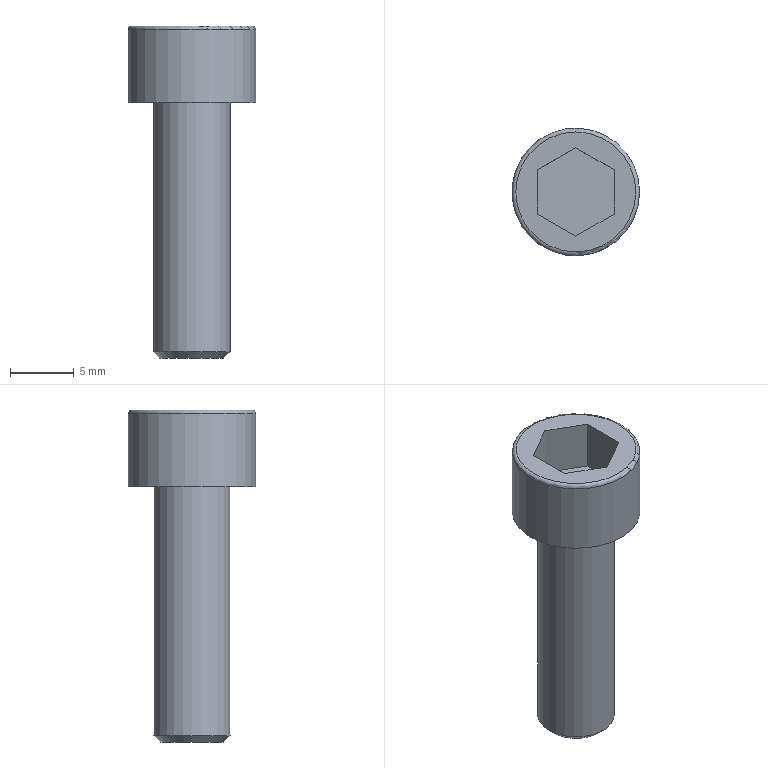Part | STEP file | 200 mesh_id994_x | 1 solid | 14 faces | box 10 x 10 x 26 mm | volume 909.194 mm3 | plane 10 | cylinder 2 | torus 1 | cone 1 | commonest cylinder face diameters 6 x1 10 x1
STEP:
#1=CARTESIAN_POINT('',(-17010.884,-3930.269,-9.5));
#2=VERTEX_POINT('',#1);
#3=CARTESIAN_POINT('',(-17007.884,-3930.269,-9.5));
#4=DIRECTION('',(0.,0.,1.));
#5=DIRECTION('',(-1.,0.,0.));
#6=AXIS2_PLACEMENT_3D('',#3,#4,#5);
#7=CIRCLE('',#6,3.);
#8=EDGE_CURVE('',#2,#2,#7,.T.);
#9=ORIENTED_EDGE('',*,*,#8,.T.);
#10=EDGE_LOOP('',(#9));
#11=FACE_BOUND('',#10,.T.);
#12=CARTESIAN_POINT('',(-17010.884,-3930.269,10.));
#13=VERTEX_POINT('',#12);
#14=CARTESIAN_POINT('',(-17007.884,-3930.269,10.));
#15=DIRECTION('',(0.,0.,1.));
#16=DIRECTION('',(-1.,0.,0.));
#17=AXIS2_PLACEMENT_3D('',#14,#15,#16);
#18=CIRCLE('',#17,3.);
#19=EDGE_CURVE('',#13,#13,#18,.T.);
#20=ORIENTED_EDGE('',*,*,#19,.F.);
#21=EDGE_LOOP('',(#20));
#22=FACE_BOUND('',#21,.T.);
#23=CARTESIAN_POINT('',(-17007.884,-3930.269,10.));
#24=DIRECTION('',(0.,0.,-1.));
#25=DIRECTION('',(1.,0.,0.));
#26=AXIS2_PLACEMENT_3D('',#23,#24,#25);
#27=CYLINDRICAL_SURFACE('',#26,3.);
#28=ADVANCED_FACE('',(#11,#22),#27,.T.);
#29=CARTESIAN_POINT('',(-17003.184,-3930.269,16.));
#30=VERTEX_POINT('',#29);
#31=CARTESIAN_POINT('',(-17007.884,-3930.269,16.));
#32=DIRECTION('',(0.,0.,1.));
#33=DIRECTION('',(1.,0.,0.));
#34=AXIS2_PLACEMENT_3D('',#31,#32,#33);
#35=CIRCLE('',#34,4.7);
#36=EDGE_CURVE('',#30,#30,#35,.T.);
#37=ORIENTED_EDGE('',*,*,#36,.T.);
#38=EDGE_LOOP('',(#37));
#39=FACE_BOUND('',#38,.T.);
#40=CARTESIAN_POINT('',(-17010.884,-3928.537,16.));
#41=VERTEX_POINT('',#40);
#42=CARTESIAN_POINT('',(-17010.884,-3932.001,16.));
#43=VERTEX_POINT('',#42);
#44=CARTESIAN_POINT('',(-17010.884,-3928.537,16.));
#45=DIRECTION('',(0.,-1.,0.));
#46=VECTOR('',#45,1.);
#47=LINE('',#44,#46);
#48=EDGE_CURVE('',#41,#43,#47,.T.);
#49=ORIENTED_EDGE('',*,*,#48,.F.);
#50=CARTESIAN_POINT('',(-17007.884,-3926.805,16.));
#51=VERTEX_POINT('',#50);
#52=CARTESIAN_POINT('',(-17007.884,-3926.805,16.));
#53=DIRECTION('',(-0.866,-0.5,0.));
#54=VECTOR('',#53,1.);
#55=LINE('',#52,#54);
#56=EDGE_CURVE('',#51,#41,#55,.T.);
#57=ORIENTED_EDGE('',*,*,#56,.F.);
#58=CARTESIAN_POINT('',(-17004.884,-3928.537,16.));
#59=VERTEX_POINT('',#58);
#60=CARTESIAN_POINT('',(-17004.884,-3928.537,16.));
#61=DIRECTION('',(-0.866,0.5,0.));
#62=VECTOR('',#61,1.);
#63=LINE('',#60,#62);
#64=EDGE_CURVE('',#59,#51,#63,.T.);
#65=ORIENTED_EDGE('',*,*,#64,.F.);
#66=CARTESIAN_POINT('',(-17004.884,-3932.001,16.));
#67=VERTEX_POINT('',#66);
#68=CARTESIAN_POINT('',(-17004.884,-3932.001,16.));
#69=DIRECTION('',(0.,1.,0.));
#70=VECTOR('',#69,1.);
#71=LINE('',#68,#70);
#72=EDGE_CURVE('',#67,#59,#71,.T.);
#73=ORIENTED_EDGE('',*,*,#72,.F.);
#74=CARTESIAN_POINT('',(-17007.884,-3933.733,16.));
#75=VERTEX_POINT('',#74);
#76=CARTESIAN_POINT('',(-17007.884,-3933.733,16.));
#77=DIRECTION('',(0.866,0.5,0.));
#78=VECTOR('',#77,1.);
#79=LINE('',#76,#78);
#80=EDGE_CURVE('',#75,#67,#79,.T.);
#81=ORIENTED_EDGE('',*,*,#80,.F.);
#82=CARTESIAN_POINT('',(-17010.884,-3932.001,16.));
#83=DIRECTION('',(0.866,-0.5,0.));
#84=VECTOR('',#83,1.);
#85=LINE('',#82,#84);
#86=EDGE_CURVE('',#43,#75,#85,.T.);
#87=ORIENTED_EDGE('',*,*,#86,.F.);
#88=EDGE_LOOP('',(#49,#57,#65,#73,#81,#87));
#89=FACE_BOUND('',#88,.T.);
#90=CARTESIAN_POINT('',(-17007.884,-3930.269,16.));
#91=DIRECTION('',(0.,0.,1.));
#92=DIRECTION('',(1.,0.,0.));
#93=AXIS2_PLACEMENT_3D('',#90,#91,#92);
#94=PLANE('',#93);
#95=ADVANCED_FACE('',(#39,#89),#94,.T.);
#96=ORIENTED_EDGE('',*,*,#19,.T.);
#97=EDGE_LOOP('',(#96));
#98=FACE_BOUND('',#97,.T.);
#99=CARTESIAN_POINT('',(-17002.884,-3930.269,10.));
#100=VERTEX_POINT('',#99);
#101=CARTESIAN_POINT('',(-17007.884,-3930.269,10.));
#102=DIRECTION('',(0.,0.,1.));
#103=DIRECTION('',(1.,0.,0.));
#104=AXIS2_PLACEMENT_3D('',#101,#102,#103);
#105=CIRCLE('',#104,5.);
#106=EDGE_CURVE('',#100,#100,#105,.T.);
#107=ORIENTED_EDGE('',*,*,#106,.F.);
#108=EDGE_LOOP('',(#107));
#109=FACE_BOUND('',#108,.T.);
#110=CARTESIAN_POINT('',(-17007.884,-3930.269,10.));
#111=DIRECTION('',(0.,0.,-1.));
#112=DIRECTION('',(-1.,0.,0.));
#113=AXIS2_PLACEMENT_3D('',#110,#111,#112);
#114=PLANE('',#113);
#115=ADVANCED_FACE('',(#98,#109),#114,.T.);
#116=CARTESIAN_POINT('',(-17002.884,-3930.269,15.7));
#117=VERTEX_POINT('',#116);
#118=CARTESIAN_POINT('',(-17007.884,-3930.269,15.7));
#119=DIRECTION('',(0.,0.,-1.));
#120=DIRECTION('',(1.,0.,0.));
#121=AXIS2_PLACEMENT_3D('',#118,#119,#120);
#122=CIRCLE('',#121,5.);
#123=EDGE_CURVE('',#117,#117,#122,.T.);
#124=ORIENTED_EDGE('',*,*,#123,.T.);
#125=EDGE_LOOP('',(#124));
#126=FACE_BOUND('',#125,.T.);
#127=ORIENTED_EDGE('',*,*,#106,.T.);
#128=EDGE_LOOP('',(#127));
#129=FACE_BOUND('',#128,.T.);
#130=CARTESIAN_POINT('',(-17007.884,-3930.269,10.));
#131=DIRECTION('',(0.,0.,1.));
#132=DIRECTION('',(1.,0.,0.));
#133=AXIS2_PLACEMENT_3D('',#130,#131,#132);
#134=CYLINDRICAL_SURFACE('',#133,5.);
#135=ADVANCED_FACE('',(#126,#129),#134,.T.);
#136=CARTESIAN_POINT('',(-17010.884,-3932.001,12.));
#137=VERTEX_POINT('',#136);
#138=CARTESIAN_POINT('',(-17010.884,-3928.537,12.));
#139=VERTEX_POINT('',#138);
#140=CARTESIAN_POINT('',(-17010.884,-3928.537,12.));
#141=DIRECTION('',(0.,1.,0.));
#142=VECTOR('',#141,1.);
#143=LINE('',#140,#142);
#144=EDGE_CURVE('',#137,#139,#143,.T.);
#145=ORIENTED_EDGE('',*,*,#144,.T.);
#146=CARTESIAN_POINT('',(-17010.884,-3928.537,16.));
#147=DIRECTION('',(0.,0.,1.));
#148=VECTOR('',#147,1.);
#149=LINE('',#146,#148);
#150=EDGE_CURVE('',#139,#41,#149,.T.);
#151=ORIENTED_EDGE('',*,*,#150,.T.);
#152=ORIENTED_EDGE('',*,*,#48,.T.);
#153=CARTESIAN_POINT('',(-17010.884,-3932.001,16.));
#154=DIRECTION('',(0.,0.,1.));
#155=VECTOR('',#154,1.);
#156=LINE('',#153,#155);
#157=EDGE_CURVE('',#137,#43,#156,.T.);
#158=ORIENTED_EDGE('',*,*,#157,.F.);
#159=EDGE_LOOP('',(#145,#151,#152,#158));
#160=FACE_OUTER_BOUND('',#159,.T.);
#161=CARTESIAN_POINT('',(-17010.884,-3928.537,16.));
#162=DIRECTION('',(1.,0.,0.));
#163=DIRECTION('',(0.,0.,-1.));
#164=AXIS2_PLACEMENT_3D('',#161,#162,#163);
#165=PLANE('',#164);
#166=ADVANCED_FACE('',(#160),#165,.T.);
#167=CARTESIAN_POINT('',(-17007.884,-3933.733,12.));
#168=VERTEX_POINT('',#167);
#169=CARTESIAN_POINT('',(-17010.884,-3932.001,12.));
#170=DIRECTION('',(-0.866,0.5,0.));
#171=VECTOR('',#170,1.);
#172=LINE('',#169,#171);
#173=EDGE_CURVE('',#168,#137,#172,.T.);
#174=ORIENTED_EDGE('',*,*,#173,.T.);
#175=ORIENTED_EDGE('',*,*,#157,.T.);
#176=ORIENTED_EDGE('',*,*,#86,.T.);
#177=CARTESIAN_POINT('',(-17007.884,-3933.733,16.));
#178=DIRECTION('',(0.,0.,1.));
#179=VECTOR('',#178,1.);
#180=LINE('',#177,#179);
#181=EDGE_CURVE('',#168,#75,#180,.T.);
#182=ORIENTED_EDGE('',*,*,#181,.F.);
#183=EDGE_LOOP('',(#174,#175,#176,#182));
#184=FACE_OUTER_BOUND('',#183,.T.);
#185=CARTESIAN_POINT('',(-17010.884,-3932.001,16.));
#186=DIRECTION('',(0.5,0.866,0.));
#187=DIRECTION('',(-0.866,0.5,0.));
#188=AXIS2_PLACEMENT_3D('',#185,#186,#187);
#189=PLANE('',#188);
#190=ADVANCED_FACE('',(#184),#189,.T.);
#191=CARTESIAN_POINT('',(-17004.884,-3932.001,12.));
#192=VERTEX_POINT('',#191);
#193=CARTESIAN_POINT('',(-17007.884,-3933.733,12.));
#194=DIRECTION('',(-0.866,-0.5,0.));
#195=VECTOR('',#194,1.);
#196=LINE('',#193,#195);
#197=EDGE_CURVE('',#192,#168,#196,.T.);
#198=ORIENTED_EDGE('',*,*,#197,.T.);
#199=ORIENTED_EDGE('',*,*,#181,.T.);
#200=ORIENTED_EDGE('',*,*,#80,.T.);
#201=CARTESIAN_POINT('',(-17004.884,-3932.001,16.));
#202=DIRECTION('',(0.,0.,1.));
#203=VECTOR('',#202,1.);
#204=LINE('',#201,#203);
#205=EDGE_CURVE('',#192,#67,#204,.T.);
#206=ORIENTED_EDGE('',*,*,#205,.F.);
#207=EDGE_LOOP('',(#198,#199,#200,#206));
#208=FACE_OUTER_BOUND('',#207,.T.);
#209=CARTESIAN_POINT('',(-17007.884,-3933.733,16.));
#210=DIRECTION('',(-0.5,0.866,0.));
#211=DIRECTION('',(-0.866,-0.5,0.));
#212=AXIS2_PLACEMENT_3D('',#209,#210,#211);
#213=PLANE('',#212);
#214=ADVANCED_FACE('',(#208),#213,.T.);
#215=CARTESIAN_POINT('',(-17004.884,-3928.537,12.));
#216=VERTEX_POINT('',#215);
#217=CARTESIAN_POINT('',(-17004.884,-3932.001,12.));
#218=DIRECTION('',(0.,-1.,0.));
#219=VECTOR('',#218,1.);
#220=LINE('',#217,#219);
#221=EDGE_CURVE('',#216,#192,#220,.T.);
#222=ORIENTED_EDGE('',*,*,#221,.T.);
#223=ORIENTED_EDGE('',*,*,#205,.T.);
#224=ORIENTED_EDGE('',*,*,#72,.T.);
#225=CARTESIAN_POINT('',(-17004.884,-3928.537,16.));
#226=DIRECTION('',(0.,0.,1.));
#227=VECTOR('',#226,1.);
#228=LINE('',#225,#227);
#229=EDGE_CURVE('',#216,#59,#228,.T.);
#230=ORIENTED_EDGE('',*,*,#229,.F.);
#231=EDGE_LOOP('',(#222,#223,#224,#230));
#232=FACE_OUTER_BOUND('',#231,.T.);
#233=CARTESIAN_POINT('',(-17004.884,-3932.001,16.));
#234=DIRECTION('',(-1.,0.,0.));
#235=DIRECTION('',(0.,0.,1.));
#236=AXIS2_PLACEMENT_3D('',#233,#234,#235);
#237=PLANE('',#236);
#238=ADVANCED_FACE('',(#232),#237,.T.);
#239=CARTESIAN_POINT('',(-17007.884,-3926.805,12.));
#240=VERTEX_POINT('',#239);
#241=CARTESIAN_POINT('',(-17004.884,-3928.537,12.));
#242=DIRECTION('',(0.866,-0.5,0.));
#243=VECTOR('',#242,1.);
#244=LINE('',#241,#243);
#245=EDGE_CURVE('',#240,#216,#244,.T.);
#246=ORIENTED_EDGE('',*,*,#245,.T.);
#247=ORIENTED_EDGE('',*,*,#229,.T.);
#248=ORIENTED_EDGE('',*,*,#64,.T.);
#249=CARTESIAN_POINT('',(-17007.884,-3926.805,16.));
#250=DIRECTION('',(0.,0.,1.));
#251=VECTOR('',#250,1.);
#252=LINE('',#249,#251);
#253=EDGE_CURVE('',#240,#51,#252,.T.);
#254=ORIENTED_EDGE('',*,*,#253,.F.);
#255=EDGE_LOOP('',(#246,#247,#248,#254));
#256=FACE_OUTER_BOUND('',#255,.T.);
#257=CARTESIAN_POINT('',(-17004.884,-3928.537,16.));
#258=DIRECTION('',(-0.5,-0.866,0.));
#259=DIRECTION('',(0.866,-0.5,0.));
#260=AXIS2_PLACEMENT_3D('',#257,#258,#259);
#261=PLANE('',#260);
#262=ADVANCED_FACE('',(#256),#261,.T.);
#263=CARTESIAN_POINT('',(-17007.884,-3926.805,12.));
#264=DIRECTION('',(0.866,0.5,0.));
#265=VECTOR('',#264,1.);
#266=LINE('',#263,#265);
#267=EDGE_CURVE('',#139,#240,#266,.T.);
#268=ORIENTED_EDGE('',*,*,#267,.T.);
#269=ORIENTED_EDGE('',*,*,#253,.T.);
#270=ORIENTED_EDGE('',*,*,#56,.T.);
#271=ORIENTED_EDGE('',*,*,#150,.F.);
#272=EDGE_LOOP('',(#268,#269,#270,#271));
#273=FACE_OUTER_BOUND('',#272,.T.);
#274=CARTESIAN_POINT('',(-17007.884,-3926.805,16.));
#275=DIRECTION('',(0.5,-0.866,0.));
#276=DIRECTION('',(0.866,0.5,0.));
#277=AXIS2_PLACEMENT_3D('',#274,#275,#276);
#278=PLANE('',#277);
#279=ADVANCED_FACE('',(#273),#278,.T.);
#280=ORIENTED_EDGE('',*,*,#144,.F.);
#281=ORIENTED_EDGE('',*,*,#173,.F.);
#282=ORIENTED_EDGE('',*,*,#197,.F.);
#283=ORIENTED_EDGE('',*,*,#221,.F.);
#284=ORIENTED_EDGE('',*,*,#245,.F.);
#285=ORIENTED_EDGE('',*,*,#267,.F.);
#286=EDGE_LOOP('',(#280,#281,#282,#283,#284,#285));
#287=FACE_OUTER_BOUND('',#286,.T.);
#288=CARTESIAN_POINT('',(-298.198,240.,12.));
#289=DIRECTION('',(0.,0.,1.));
#290=DIRECTION('',(1.,0.,0.));
#291=AXIS2_PLACEMENT_3D('',#288,#289,#290);
#292=PLANE('',#291);
#293=ADVANCED_FACE('',(#287),#292,.T.);
#294=ORIENTED_EDGE('',*,*,#36,.F.);
#295=EDGE_LOOP('',(#294));
#296=FACE_BOUND('',#295,.T.);
#297=ORIENTED_EDGE('',*,*,#123,.F.);
#298=EDGE_LOOP('',(#297));
#299=FACE_BOUND('',#298,.T.);
#300=CARTESIAN_POINT('',(-17007.884,-3930.269,15.7));
#301=DIRECTION('',(0.,0.,1.));
#302=DIRECTION('',(1.,0.,0.));
#303=AXIS2_PLACEMENT_3D('',#300,#301,#302);
#304=TOROIDAL_SURFACE('',#303,4.7,0.3);
#305=ADVANCED_FACE('',(#296,#299),#304,.T.);
#306=CARTESIAN_POINT('',(-17010.384,-3930.269,-10.));
#307=VERTEX_POINT('',#306);
#308=CARTESIAN_POINT('',(-17007.884,-3930.269,-10.));
#309=DIRECTION('',(0.,0.,-1.));
#310=DIRECTION('',(-1.,0.,0.));
#311=AXIS2_PLACEMENT_3D('',#308,#309,#310);
#312=CIRCLE('',#311,2.5);
#313=EDGE_CURVE('',#307,#307,#312,.T.);
#314=ORIENTED_EDGE('',*,*,#313,.T.);
#315=EDGE_LOOP('',(#314));
#316=FACE_OUTER_BOUND('',#315,.T.);
#317=CARTESIAN_POINT('',(-17007.884,-3930.269,-10.));
#318=DIRECTION('',(0.,0.,-1.));
#319=DIRECTION('',(-1.,0.,0.));
#320=AXIS2_PLACEMENT_3D('',#317,#318,#319);
#321=PLANE('',#320);
#322=ADVANCED_FACE('',(#316),#321,.T.);
#323=ORIENTED_EDGE('',*,*,#313,.F.);
#324=EDGE_LOOP('',(#323));
#325=FACE_BOUND('',#324,.T.);
#326=ORIENTED_EDGE('',*,*,#8,.F.);
#327=EDGE_LOOP('',(#326));
#328=FACE_BOUND('',#327,.T.);
#329=CARTESIAN_POINT('',(-17007.884,-3930.269,-9.5));
#330=DIRECTION('',(0.,0.,1.));
#331=DIRECTION('',(1.,0.,0.));
#332=AXIS2_PLACEMENT_3D('',#329,#330,#331);
#333=CONICAL_SURFACE('',#332,3.,45.);
#334=ADVANCED_FACE('',(#325,#328),#333,.T.);
#335=CLOSED_SHELL('',(#28,#95,#115,#135,#166,#190,#214,#238,#262,#279,#293,#305,#322,#334));
#336=MANIFOLD_SOLID_BREP('',#335);
#337=(LENGTH_UNIT()NAMED_UNIT(*)SI_UNIT(.MILLI.,.METRE.));
#338=UNCERTAINTY_MEASURE_WITH_UNIT(LENGTH_MEASURE(0.00002),#337,'','');
#339=(NAMED_UNIT(*)PLANE_ANGLE_UNIT()SI_UNIT($,.RADIAN.));
#340=PLANE_ANGLE_MEASURE_WITH_UNIT(PLANE_ANGLE_MEASURE(0.01745),#339);
#341=DIMENSIONAL_EXPONENTS(0.,0.,0.,0.,0.,0.,0.);
#342=(CONVERSION_BASED_UNIT('DEGREE',#340)NAMED_UNIT(#341)PLANE_ANGLE_UNIT());
#343=(NAMED_UNIT(*)SI_UNIT($,.STERADIAN.)SOLID_ANGLE_UNIT());
#344=(GEOMETRIC_REPRESENTATION_CONTEXT(3)GLOBAL_UNCERTAINTY_ASSIGNED_CONTEXT((#338))GLOBAL_UNIT_ASSIGNED_CONTEXT((#337,#342,#343))REPRESENTATION_CONTEXT('',''));
#345=ADVANCED_BREP_SHAPE_REPRESENTATION('',(#336),#344);